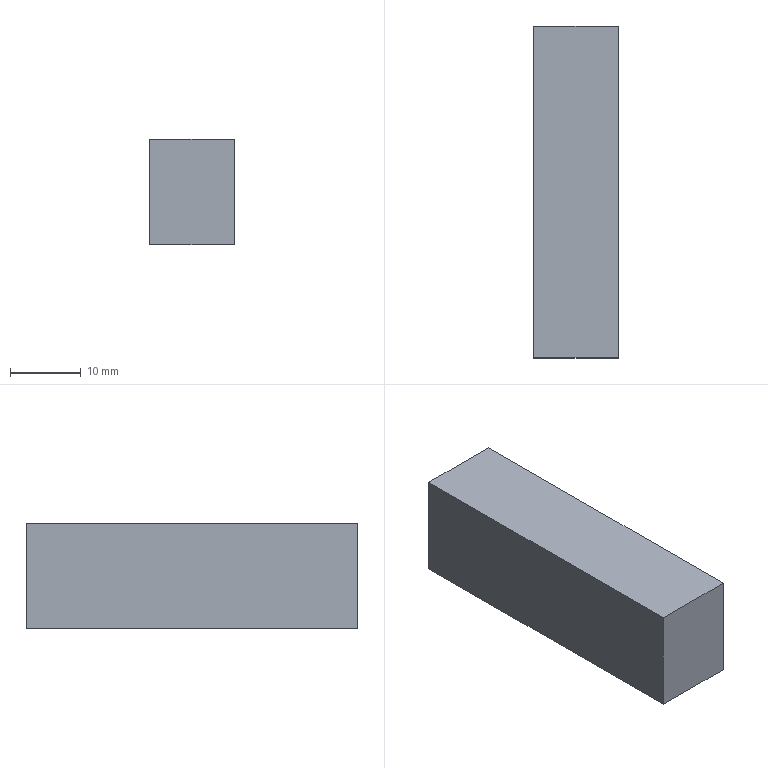Part | NX | features solid 2 | 1 solid | 6 faces | box 12 x 47 x 15 mm | volume 8460 mm3 | plane 6
STEP:
#1=CARTESIAN_POINT('',(-423.,722.,-15.));
#2=VERTEX_POINT('',#1);
#3=CARTESIAN_POINT('',(-435.,722.,-15.));
#4=VERTEX_POINT('',#3);
#5=CARTESIAN_POINT('',(-284.,722.,-15.));
#6=DIRECTION('',(-1.,0.,0.));
#7=VECTOR('',#6,1000.);
#8=LINE('',#5,#7);
#9=EDGE_CURVE('',#2,#4,#8,.T.);
#10=ORIENTED_EDGE('',*,*,#9,.F.);
#11=CARTESIAN_POINT('',(-423.,722.,-30.));
#12=VERTEX_POINT('',#11);
#13=CARTESIAN_POINT('',(-423.,722.,-30.));
#14=DIRECTION('',(0.,0.,1.));
#15=VECTOR('',#14,1000.);
#16=LINE('',#13,#15);
#17=EDGE_CURVE('',#12,#2,#16,.T.);
#18=ORIENTED_EDGE('',*,*,#17,.F.);
#19=CARTESIAN_POINT('',(-435.,722.,-30.));
#20=VERTEX_POINT('',#19);
#21=CARTESIAN_POINT('',(-284.,722.,-30.));
#22=DIRECTION('',(-1.,0.,0.));
#23=VECTOR('',#22,1000.);
#24=LINE('',#21,#23);
#25=EDGE_CURVE('',#12,#20,#24,.T.);
#26=ORIENTED_EDGE('',*,*,#25,.T.);
#27=CARTESIAN_POINT('',(-435.,722.,59.523));
#28=DIRECTION('',(0.,0.,1.));
#29=VECTOR('',#28,1000.);
#30=LINE('',#27,#29);
#31=EDGE_CURVE('',#20,#4,#30,.T.);
#32=ORIENTED_EDGE('',*,*,#31,.T.);
#33=EDGE_LOOP('',(#10,#18,#26,#32));
#34=FACE_BOUND('',#33,.T.);
#35=CARTESIAN_POINT('',(-284.,722.,59.523));
#36=DIRECTION('',(0.,-1.,0.));
#37=DIRECTION('',(-1.,0.,0.));
#38=AXIS2_PLACEMENT_3D('',#35,#36,#37);
#39=PLANE('',#38);
#40=ADVANCED_FACE('',(#34),#39,.F.);
#41=ORIENTED_EDGE('',*,*,#9,.T.);
#42=CARTESIAN_POINT('',(-435.,675.,-15.));
#43=VERTEX_POINT('',#42);
#44=CARTESIAN_POINT('',(-435.,842.,-15.));
#45=DIRECTION('',(0.,1.,0.));
#46=VECTOR('',#45,1000.);
#47=LINE('',#44,#46);
#48=EDGE_CURVE('',#43,#4,#47,.T.);
#49=ORIENTED_EDGE('',*,*,#48,.F.);
#50=CARTESIAN_POINT('',(-423.,675.,-15.));
#51=VERTEX_POINT('',#50);
#52=CARTESIAN_POINT('',(-435.,675.,-15.));
#53=DIRECTION('',(-1.,0.,0.));
#54=VECTOR('',#53,1000.);
#55=LINE('',#52,#54);
#56=EDGE_CURVE('',#43,#51,#55,.F.);
#57=ORIENTED_EDGE('',*,*,#56,.T.);
#58=CARTESIAN_POINT('',(-423.,736.,-15.));
#59=DIRECTION('',(0.,1.,0.));
#60=VECTOR('',#59,1000.);
#61=LINE('',#58,#60);
#62=EDGE_CURVE('',#2,#51,#61,.F.);
#63=ORIENTED_EDGE('',*,*,#62,.F.);
#64=EDGE_LOOP('',(#41,#49,#57,#63));
#65=FACE_BOUND('',#64,.T.);
#66=CARTESIAN_POINT('',(-228.,767.,-15.));
#67=DIRECTION('',(0.,0.,1.));
#68=DIRECTION('',(0.,1.,0.));
#69=AXIS2_PLACEMENT_3D('',#66,#67,#68);
#70=PLANE('',#69);
#71=ADVANCED_FACE('',(#65),#70,.T.);
#72=CARTESIAN_POINT('',(-435.,675.,-30.));
#73=VERTEX_POINT('',#72);
#74=CARTESIAN_POINT('',(-435.,842.,-30.));
#75=DIRECTION('',(0.,1.,0.));
#76=VECTOR('',#75,1000.);
#77=LINE('',#74,#76);
#78=EDGE_CURVE('',#73,#20,#77,.T.);
#79=ORIENTED_EDGE('',*,*,#78,.T.);
#80=ORIENTED_EDGE('',*,*,#25,.F.);
#81=CARTESIAN_POINT('',(-423.,675.,-30.));
#82=VERTEX_POINT('',#81);
#83=CARTESIAN_POINT('',(-423.,736.,-30.));
#84=DIRECTION('',(0.,1.,0.));
#85=VECTOR('',#84,1000.);
#86=LINE('',#83,#85);
#87=EDGE_CURVE('',#12,#82,#86,.F.);
#88=ORIENTED_EDGE('',*,*,#87,.T.);
#89=CARTESIAN_POINT('',(-228.,675.,-30.));
#90=DIRECTION('',(1.,0.,0.));
#91=VECTOR('',#90,1000.);
#92=LINE('',#89,#91);
#93=EDGE_CURVE('',#73,#82,#92,.T.);
#94=ORIENTED_EDGE('',*,*,#93,.F.);
#95=EDGE_LOOP('',(#79,#80,#88,#94));
#96=FACE_BOUND('',#95,.T.);
#97=CARTESIAN_POINT('',(-228.,767.,-30.));
#98=DIRECTION('',(0.,0.,1.));
#99=DIRECTION('',(0.,1.,0.));
#100=AXIS2_PLACEMENT_3D('',#97,#98,#99);
#101=PLANE('',#100);
#102=ADVANCED_FACE('',(#96),#101,.F.);
#103=ORIENTED_EDGE('',*,*,#87,.F.);
#104=ORIENTED_EDGE('',*,*,#17,.T.);
#105=ORIENTED_EDGE('',*,*,#62,.T.);
#106=CARTESIAN_POINT('',(-423.,675.,-30.));
#107=DIRECTION('',(0.,0.,1.));
#108=VECTOR('',#107,1000.);
#109=LINE('',#106,#108);
#110=EDGE_CURVE('',#82,#51,#109,.T.);
#111=ORIENTED_EDGE('',*,*,#110,.F.);
#112=EDGE_LOOP('',(#103,#104,#105,#111));
#113=FACE_BOUND('',#112,.T.);
#114=CARTESIAN_POINT('',(-423.,736.,-30.));
#115=DIRECTION('',(-1.,0.,0.));
#116=DIRECTION('',(0.,0.,1.));
#117=AXIS2_PLACEMENT_3D('',#114,#115,#116);
#118=PLANE('',#117);
#119=ADVANCED_FACE('',(#113),#118,.F.);
#120=ORIENTED_EDGE('',*,*,#48,.T.);
#121=ORIENTED_EDGE('',*,*,#31,.F.);
#122=ORIENTED_EDGE('',*,*,#78,.F.);
#123=CARTESIAN_POINT('',(-435.,675.,59.523));
#124=DIRECTION('',(0.,0.,-1.));
#125=VECTOR('',#124,1000.);
#126=LINE('',#123,#125);
#127=EDGE_CURVE('',#43,#73,#126,.T.);
#128=ORIENTED_EDGE('',*,*,#127,.F.);
#129=EDGE_LOOP('',(#120,#121,#122,#128));
#130=FACE_BOUND('',#129,.T.);
#131=CARTESIAN_POINT('',(-435.,842.,59.523));
#132=DIRECTION('',(1.,0.,0.));
#133=DIRECTION('',(0.,-1.,0.));
#134=AXIS2_PLACEMENT_3D('',#131,#132,#133);
#135=PLANE('',#134);
#136=ADVANCED_FACE('',(#130),#135,.F.);
#137=ORIENTED_EDGE('',*,*,#93,.T.);
#138=ORIENTED_EDGE('',*,*,#110,.T.);
#139=ORIENTED_EDGE('',*,*,#56,.F.);
#140=ORIENTED_EDGE('',*,*,#127,.T.);
#141=EDGE_LOOP('',(#137,#138,#139,#140));
#142=FACE_BOUND('',#141,.T.);
#143=CARTESIAN_POINT('',(-435.,675.,-15.));
#144=DIRECTION('',(0.,1.,0.));
#145=DIRECTION('',(0.,0.,1.));
#146=AXIS2_PLACEMENT_3D('',#143,#144,#145);
#147=PLANE('',#146);
#148=ADVANCED_FACE('',(#142),#147,.F.);
#149=CLOSED_SHELL('',(#40,#71,#102,#119,#136,#148));
#150=MANIFOLD_SOLID_BREP('',#149);
#151=(LENGTH_UNIT()NAMED_UNIT(*)SI_UNIT(.MILLI.,.METRE.));
#152=UNCERTAINTY_MEASURE_WITH_UNIT(LENGTH_MEASURE(0.00001),#151,'','');
#153=(NAMED_UNIT(*)PLANE_ANGLE_UNIT()SI_UNIT($,.RADIAN.));
#154=(NAMED_UNIT(*)SI_UNIT($,.STERADIAN.)SOLID_ANGLE_UNIT());
#155=(GEOMETRIC_REPRESENTATION_CONTEXT(3)GLOBAL_UNCERTAINTY_ASSIGNED_CONTEXT((#152))GLOBAL_UNIT_ASSIGNED_CONTEXT((#151,#153,#154))REPRESENTATION_CONTEXT('',''));
#156=ADVANCED_BREP_SHAPE_REPRESENTATION('',(#150),#155);